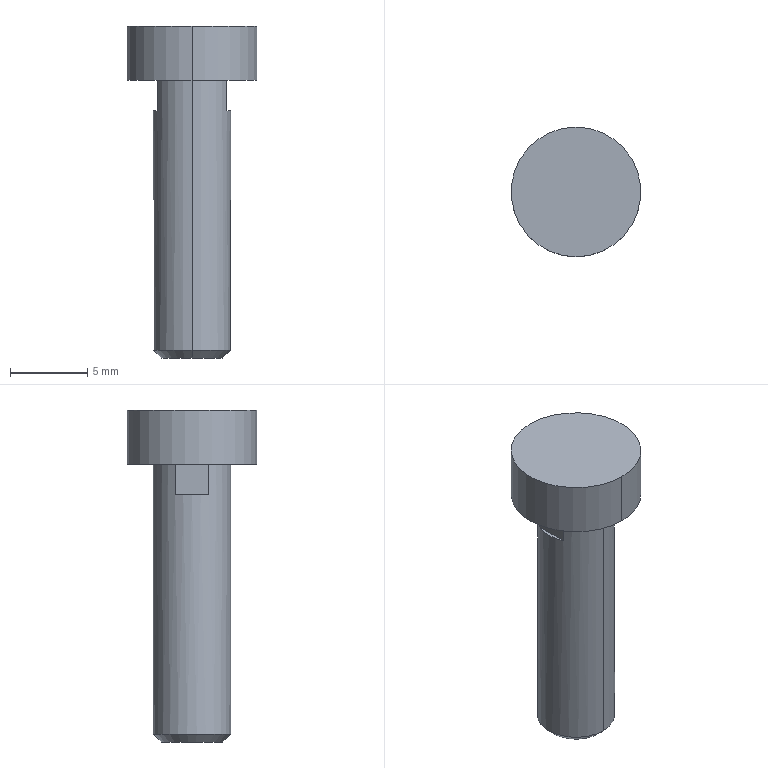Part | STEP file | M5 screw_default | 1 solid | 13 faces | box 8.4 x 8.4 x 21.5 mm | volume 544.09 mm3 | plane 7 | cylinder 4 | cone 2 | commonest cylinder face diameters 5 x2 8.4 x2
STEP:
#1=CARTESIAN_POINT('',(0.,0.,0.));
#2=DIRECTION('',(0.,0.,1.));
#3=DIRECTION('',(1.,0.,0.));
#4=AXIS2_PLACEMENT_3D('',#1,#2,#3);
#5=CARTESIAN_POINT('',(0.,2.,-3.));
#6=VERTEX_POINT('',#5);
#7=CARTESIAN_POINT('',(0.,-2.,-3.));
#8=VERTEX_POINT('',#7);
#9=CARTESIAN_POINT('',(0.,0.,-3.));
#10=DIRECTION('',(0.,0.,-1.));
#11=DIRECTION('',(-1.,0.,0.));
#12=AXIS2_PLACEMENT_3D('',#9,#10,#11);
#13=CIRCLE('',#12,2.);
#14=CARTESIAN_POINT('',(0.,0.,-3.));
#15=DIRECTION('',(0.,0.,1.));
#16=DIRECTION('',(0.,-1.,0.));
#17=AXIS2_PLACEMENT_3D('',#14,#15,#16);
#18=CONICAL_SURFACE('',#17,2.,0.7854);
#19=CARTESIAN_POINT('',(4.712,0.));
#20=DIRECTION('',(-1.,0.));
#21=VECTOR('',#20,1.);
#22=LINE('',#19,#21);
#23=(GEOMETRIC_REPRESENTATION_CONTEXT(2)PARAMETRIC_REPRESENTATION_CONTEXT()REPRESENTATION_CONTEXT('',''));
#24=DEFINITIONAL_REPRESENTATION('',(#22),#23);
#25=PCURVE('',#18,#24);
#26=CARTESIAN_POINT('',(0.,0.,-3.));
#27=DIRECTION('',(0.,0.,-1.));
#28=DIRECTION('',(-1.,0.,0.));
#29=AXIS2_PLACEMENT_3D('',#26,#27,#28);
#30=PLANE('',#29);
#31=CARTESIAN_POINT('',(0.,0.));
#32=DIRECTION('',(1.,0.));
#33=AXIS2_PLACEMENT_2D('',#31,#32);
#34=CIRCLE('',#33,2.);
#35=(GEOMETRIC_REPRESENTATION_CONTEXT(2)PARAMETRIC_REPRESENTATION_CONTEXT()REPRESENTATION_CONTEXT('',''));
#36=DEFINITIONAL_REPRESENTATION('',(#34),#35);
#37=PCURVE('',#30,#36);
#38=SURFACE_CURVE('',#13,(#25,#37),.PCURVE_S1.);
#39=EDGE_CURVE('',#6,#8,#38,.T.);
#40=ORIENTED_EDGE('',*,*,#39,.F.);
#41=CARTESIAN_POINT('',(0.,2.5,-2.5));
#42=VERTEX_POINT('',#41);
#43=CARTESIAN_POINT('',(0.,2.,-3.));
#44=DIRECTION('',(0.,0.7071,0.7071));
#45=VECTOR('',#44,1.);
#46=LINE('',#43,#45);
#47=CARTESIAN_POINT('',(3.142,0.));
#48=DIRECTION('',(0.,1.));
#49=VECTOR('',#48,1.);
#50=LINE('',#47,#49);
#51=(GEOMETRIC_REPRESENTATION_CONTEXT(2)PARAMETRIC_REPRESENTATION_CONTEXT()REPRESENTATION_CONTEXT('',''));
#52=DEFINITIONAL_REPRESENTATION('',(#50),#51);
#53=PCURVE('',#18,#52);
#54=CARTESIAN_POINT('',(0.,0.,-3.));
#55=DIRECTION('',(0.,0.,1.));
#56=DIRECTION('',(0.,-1.,0.));
#57=AXIS2_PLACEMENT_3D('',#54,#55,#56);
#58=CONICAL_SURFACE('',#57,2.,0.7854);
#59=CARTESIAN_POINT('',(3.142,0.));
#60=DIRECTION('',(0.,1.));
#61=VECTOR('',#60,1.);
#62=LINE('',#59,#61);
#63=(GEOMETRIC_REPRESENTATION_CONTEXT(2)PARAMETRIC_REPRESENTATION_CONTEXT()REPRESENTATION_CONTEXT('',''));
#64=DEFINITIONAL_REPRESENTATION('',(#62),#63);
#65=PCURVE('',#58,#64);
#66=SURFACE_CURVE('',#46,(#53,#65),.PCURVE_S1.);
#67=EDGE_CURVE('',#6,#42,#66,.T.);
#68=ORIENTED_EDGE('',*,*,#67,.T.);
#69=CARTESIAN_POINT('',(0.,-2.5,-2.5));
#70=VERTEX_POINT('',#69);
#71=CARTESIAN_POINT('',(0.,0.,-2.5));
#72=DIRECTION('',(0.,0.,1.));
#73=DIRECTION('',(0.,1.,0.));
#74=AXIS2_PLACEMENT_3D('',#71,#72,#73);
#75=CIRCLE('',#74,2.5);
#76=CARTESIAN_POINT('',(-3.142,0.5));
#77=DIRECTION('',(1.,0.));
#78=VECTOR('',#77,1.);
#79=LINE('',#76,#78);
#80=(GEOMETRIC_REPRESENTATION_CONTEXT(2)PARAMETRIC_REPRESENTATION_CONTEXT()REPRESENTATION_CONTEXT('',''));
#81=DEFINITIONAL_REPRESENTATION('',(#79),#80);
#82=PCURVE('',#18,#81);
#83=CARTESIAN_POINT('',(0.,0.,15.));
#84=DIRECTION('',(0.,0.,-1.));
#85=DIRECTION('',(0.,1.,0.));
#86=AXIS2_PLACEMENT_3D('',#83,#84,#85);
#87=CYLINDRICAL_SURFACE('',#86,2.5);
#88=CARTESIAN_POINT('',(6.283,17.5));
#89=DIRECTION('',(-1.,0.));
#90=VECTOR('',#89,1.);
#91=LINE('',#88,#90);
#92=(GEOMETRIC_REPRESENTATION_CONTEXT(2)PARAMETRIC_REPRESENTATION_CONTEXT()REPRESENTATION_CONTEXT('',''));
#93=DEFINITIONAL_REPRESENTATION('',(#91),#92);
#94=PCURVE('',#87,#93);
#95=SURFACE_CURVE('',#75,(#82,#94),.PCURVE_S1.);
#96=EDGE_CURVE('',#70,#42,#95,.T.);
#97=ORIENTED_EDGE('',*,*,#96,.F.);
#98=CARTESIAN_POINT('',(0.,-2.,-3.));
#99=DIRECTION('',(0.,-0.7071,0.7071));
#100=VECTOR('',#99,1.);
#101=LINE('',#98,#100);
#102=CARTESIAN_POINT('',(0.,0.));
#103=DIRECTION('',(0.,1.));
#104=VECTOR('',#103,1.);
#105=LINE('',#102,#104);
#106=(GEOMETRIC_REPRESENTATION_CONTEXT(2)PARAMETRIC_REPRESENTATION_CONTEXT()REPRESENTATION_CONTEXT('',''));
#107=DEFINITIONAL_REPRESENTATION('',(#105),#106);
#108=PCURVE('',#18,#107);
#109=CARTESIAN_POINT('',(6.283,0.));
#110=DIRECTION('',(0.,1.));
#111=VECTOR('',#110,1.);
#112=LINE('',#109,#111);
#113=(GEOMETRIC_REPRESENTATION_CONTEXT(2)PARAMETRIC_REPRESENTATION_CONTEXT()REPRESENTATION_CONTEXT('',''));
#114=DEFINITIONAL_REPRESENTATION('',(#112),#113);
#115=PCURVE('',#58,#114);
#116=SURFACE_CURVE('',#101,(#108,#115),.PCURVE_S1.);
#117=EDGE_CURVE('',#8,#70,#116,.T.);
#118=ORIENTED_EDGE('',*,*,#117,.F.);
#119=EDGE_LOOP('',(#40,#68,#97,#118));
#120=FACE_BOUND('',#119,.T.);
#121=ADVANCED_FACE('',(#120),#18,.T.);
#122=CARTESIAN_POINT('',(0.,-2.5,15.));
#123=VERTEX_POINT('',#122);
#124=CARTESIAN_POINT('',(2.25,-1.09,15.));
#125=VERTEX_POINT('',#124);
#126=CARTESIAN_POINT('',(0.,0.,15.));
#127=DIRECTION('',(0.,0.,1.));
#128=DIRECTION('',(0.,1.,0.));
#129=AXIS2_PLACEMENT_3D('',#126,#127,#128);
#130=CIRCLE('',#129,2.5);
#131=CARTESIAN_POINT('',(6.283,0.));
#132=DIRECTION('',(-1.,0.));
#133=VECTOR('',#132,1.);
#134=LINE('',#131,#133);
#135=(GEOMETRIC_REPRESENTATION_CONTEXT(2)PARAMETRIC_REPRESENTATION_CONTEXT()REPRESENTATION_CONTEXT('',''));
#136=DEFINITIONAL_REPRESENTATION('',(#134),#135);
#137=PCURVE('',#87,#136);
#138=CARTESIAN_POINT('',(-4.25,-4.25,15.));
#139=DIRECTION('',(0.,0.,1.));
#140=DIRECTION('',(1.,0.,0.));
#141=AXIS2_PLACEMENT_3D('',#138,#139,#140);
#142=PLANE('',#141);
#143=CARTESIAN_POINT('',(4.25,4.25));
#144=DIRECTION('',(0.,1.));
#145=AXIS2_PLACEMENT_2D('',#143,#144);
#146=CIRCLE('',#145,2.5);
#147=(GEOMETRIC_REPRESENTATION_CONTEXT(2)PARAMETRIC_REPRESENTATION_CONTEXT()REPRESENTATION_CONTEXT('',''));
#148=DEFINITIONAL_REPRESENTATION('',(#146),#147);
#149=PCURVE('',#142,#148);
#150=SURFACE_CURVE('',#130,(#137,#149),.PCURVE_S1.);
#151=EDGE_CURVE('',#123,#125,#150,.T.);
#152=ORIENTED_EDGE('',*,*,#151,.F.);
#153=CARTESIAN_POINT('',(0.,-2.5,15.));
#154=DIRECTION('',(0.,0.,-1.));
#155=VECTOR('',#154,1.);
#156=LINE('',#153,#155);
#157=CARTESIAN_POINT('',(3.142,0.));
#158=DIRECTION('',(0.,1.));
#159=VECTOR('',#158,1.);
#160=LINE('',#157,#159);
#161=(GEOMETRIC_REPRESENTATION_CONTEXT(2)PARAMETRIC_REPRESENTATION_CONTEXT()REPRESENTATION_CONTEXT('',''));
#162=DEFINITIONAL_REPRESENTATION('',(#160),#161);
#163=PCURVE('',#87,#162);
#164=CARTESIAN_POINT('',(0.,0.,15.));
#165=DIRECTION('',(0.,0.,-1.));
#166=DIRECTION('',(0.,1.,0.));
#167=AXIS2_PLACEMENT_3D('',#164,#165,#166);
#168=CYLINDRICAL_SURFACE('',#167,2.5);
#169=CARTESIAN_POINT('',(3.142,0.));
#170=DIRECTION('',(0.,1.));
#171=VECTOR('',#170,1.);
#172=LINE('',#169,#171);
#173=(GEOMETRIC_REPRESENTATION_CONTEXT(2)PARAMETRIC_REPRESENTATION_CONTEXT()REPRESENTATION_CONTEXT('',''));
#174=DEFINITIONAL_REPRESENTATION('',(#172),#173);
#175=PCURVE('',#168,#174);
#176=SURFACE_CURVE('',#156,(#163,#175),.PCURVE_S1.);
#177=EDGE_CURVE('',#123,#70,#176,.T.);
#178=ORIENTED_EDGE('',*,*,#177,.T.);
#179=ORIENTED_EDGE('',*,*,#96,.T.);
#180=CARTESIAN_POINT('',(0.,2.5,15.));
#181=VERTEX_POINT('',#180);
#182=CARTESIAN_POINT('',(0.,2.5,15.));
#183=DIRECTION('',(0.,0.,-1.));
#184=VECTOR('',#183,1.);
#185=LINE('',#182,#184);
#186=CARTESIAN_POINT('',(0.,0.));
#187=DIRECTION('',(0.,1.));
#188=VECTOR('',#187,1.);
#189=LINE('',#186,#188);
#190=(GEOMETRIC_REPRESENTATION_CONTEXT(2)PARAMETRIC_REPRESENTATION_CONTEXT()REPRESENTATION_CONTEXT('',''));
#191=DEFINITIONAL_REPRESENTATION('',(#189),#190);
#192=PCURVE('',#87,#191);
#193=CARTESIAN_POINT('',(6.283,0.));
#194=DIRECTION('',(0.,1.));
#195=VECTOR('',#194,1.);
#196=LINE('',#193,#195);
#197=(GEOMETRIC_REPRESENTATION_CONTEXT(2)PARAMETRIC_REPRESENTATION_CONTEXT()REPRESENTATION_CONTEXT('',''));
#198=DEFINITIONAL_REPRESENTATION('',(#196),#197);
#199=PCURVE('',#168,#198);
#200=SURFACE_CURVE('',#185,(#192,#199),.PCURVE_S1.);
#201=EDGE_CURVE('',#181,#42,#200,.T.);
#202=ORIENTED_EDGE('',*,*,#201,.F.);
#203=CARTESIAN_POINT('',(2.25,1.09,15.));
#204=VERTEX_POINT('',#203);
#205=CARTESIAN_POINT('',(0.,0.,15.));
#206=DIRECTION('',(0.,0.,1.));
#207=DIRECTION('',(0.,1.,0.));
#208=AXIS2_PLACEMENT_3D('',#205,#206,#207);
#209=CIRCLE('',#208,2.5);
#210=CARTESIAN_POINT('',(6.283,0.));
#211=DIRECTION('',(-1.,0.));
#212=VECTOR('',#211,1.);
#213=LINE('',#210,#212);
#214=(GEOMETRIC_REPRESENTATION_CONTEXT(2)PARAMETRIC_REPRESENTATION_CONTEXT()REPRESENTATION_CONTEXT('',''));
#215=DEFINITIONAL_REPRESENTATION('',(#213),#214);
#216=PCURVE('',#87,#215);
#217=CARTESIAN_POINT('',(4.25,4.25));
#218=DIRECTION('',(0.,1.));
#219=AXIS2_PLACEMENT_2D('',#217,#218);
#220=CIRCLE('',#219,2.5);
#221=(GEOMETRIC_REPRESENTATION_CONTEXT(2)PARAMETRIC_REPRESENTATION_CONTEXT()REPRESENTATION_CONTEXT('',''));
#222=DEFINITIONAL_REPRESENTATION('',(#220),#221);
#223=PCURVE('',#142,#222);
#224=SURFACE_CURVE('',#209,(#216,#223),.PCURVE_S1.);
#225=EDGE_CURVE('',#204,#181,#224,.T.);
#226=ORIENTED_EDGE('',*,*,#225,.F.);
#227=CARTESIAN_POINT('',(2.25,1.09,13.));
#228=VERTEX_POINT('',#227);
#229=CARTESIAN_POINT('',(2.25,1.09,15.));
#230=DIRECTION('',(0.,0.,-1.));
#231=VECTOR('',#230,1.);
#232=LINE('',#229,#231);
#233=CARTESIAN_POINT('',(1.12,0.));
#234=DIRECTION('',(0.,1.));
#235=VECTOR('',#234,1.);
#236=LINE('',#233,#235);
#237=(GEOMETRIC_REPRESENTATION_CONTEXT(2)PARAMETRIC_REPRESENTATION_CONTEXT()REPRESENTATION_CONTEXT('',''));
#238=DEFINITIONAL_REPRESENTATION('',(#236),#237);
#239=PCURVE('',#87,#238);
#240=CARTESIAN_POINT('',(2.25,-9.,15.));
#241=DIRECTION('',(-1.,0.,0.));
#242=DIRECTION('',(0.,0.,1.));
#243=AXIS2_PLACEMENT_3D('',#240,#241,#242);
#244=PLANE('',#243);
#245=CARTESIAN_POINT('',(0.,10.09));
#246=DIRECTION('',(-1.,0.));
#247=VECTOR('',#246,1.);
#248=LINE('',#245,#247);
#249=(GEOMETRIC_REPRESENTATION_CONTEXT(2)PARAMETRIC_REPRESENTATION_CONTEXT()REPRESENTATION_CONTEXT('',''));
#250=DEFINITIONAL_REPRESENTATION('',(#248),#249);
#251=PCURVE('',#244,#250);
#252=SURFACE_CURVE('',#232,(#239,#251),.PCURVE_S1.);
#253=EDGE_CURVE('',#204,#228,#252,.T.);
#254=ORIENTED_EDGE('',*,*,#253,.T.);
#255=CARTESIAN_POINT('',(2.25,-1.09,13.));
#256=VERTEX_POINT('',#255);
#257=CARTESIAN_POINT('',(0.,0.,13.));
#258=DIRECTION('',(0.,0.,-1.));
#259=DIRECTION('',(-1.,0.,0.));
#260=AXIS2_PLACEMENT_3D('',#257,#258,#259);
#261=CIRCLE('',#260,2.5);
#262=CARTESIAN_POINT('',(-1.571,2.));
#263=DIRECTION('',(1.,0.));
#264=VECTOR('',#263,1.);
#265=LINE('',#262,#264);
#266=(GEOMETRIC_REPRESENTATION_CONTEXT(2)PARAMETRIC_REPRESENTATION_CONTEXT()REPRESENTATION_CONTEXT('',''));
#267=DEFINITIONAL_REPRESENTATION('',(#265),#266);
#268=PCURVE('',#87,#267);
#269=CARTESIAN_POINT('',(3.25,-9.,13.));
#270=DIRECTION('',(0.,0.,-1.));
#271=DIRECTION('',(-1.,0.,0.));
#272=AXIS2_PLACEMENT_3D('',#269,#270,#271);
#273=PLANE('',#272);
#274=CARTESIAN_POINT('',(3.25,9.));
#275=DIRECTION('',(1.,0.));
#276=AXIS2_PLACEMENT_2D('',#274,#275);
#277=CIRCLE('',#276,2.5);
#278=(GEOMETRIC_REPRESENTATION_CONTEXT(2)PARAMETRIC_REPRESENTATION_CONTEXT()REPRESENTATION_CONTEXT('',''));
#279=DEFINITIONAL_REPRESENTATION('',(#277),#278);
#280=PCURVE('',#273,#279);
#281=SURFACE_CURVE('',#261,(#268,#280),.PCURVE_S1.);
#282=EDGE_CURVE('',#228,#256,#281,.T.);
#283=ORIENTED_EDGE('',*,*,#282,.T.);
#284=CARTESIAN_POINT('',(2.25,-1.09,15.));
#285=DIRECTION('',(0.,0.,1.));
#286=VECTOR('',#285,1.);
#287=LINE('',#284,#286);
#288=CARTESIAN_POINT('',(2.022,0.));
#289=DIRECTION('',(0.,-1.));
#290=VECTOR('',#289,1.);
#291=LINE('',#288,#290);
#292=(GEOMETRIC_REPRESENTATION_CONTEXT(2)PARAMETRIC_REPRESENTATION_CONTEXT()REPRESENTATION_CONTEXT('',''));
#293=DEFINITIONAL_REPRESENTATION('',(#291),#292);
#294=PCURVE('',#87,#293);
#295=CARTESIAN_POINT('',(0.,7.91));
#296=DIRECTION('',(1.,0.));
#297=VECTOR('',#296,1.);
#298=LINE('',#295,#297);
#299=(GEOMETRIC_REPRESENTATION_CONTEXT(2)PARAMETRIC_REPRESENTATION_CONTEXT()REPRESENTATION_CONTEXT('',''));
#300=DEFINITIONAL_REPRESENTATION('',(#298),#299);
#301=PCURVE('',#244,#300);
#302=SURFACE_CURVE('',#287,(#294,#301),.PCURVE_S1.);
#303=EDGE_CURVE('',#256,#125,#302,.T.);
#304=ORIENTED_EDGE('',*,*,#303,.T.);
#305=EDGE_LOOP('',(#152,#178,#179,#202,#226,#254,#283,#304));
#306=FACE_BOUND('',#305,.T.);
#307=ADVANCED_FACE('',(#306),#87,.T.);
#308=CARTESIAN_POINT('',(0.,-4.2,18.5));
#309=VERTEX_POINT('',#308);
#310=CARTESIAN_POINT('',(0.,4.2,18.5));
#311=VERTEX_POINT('',#310);
#312=CARTESIAN_POINT('',(0.,0.,18.5));
#313=DIRECTION('',(0.,0.,1.));
#314=DIRECTION('',(0.,1.,0.));
#315=AXIS2_PLACEMENT_3D('',#312,#313,#314);
#316=CIRCLE('',#315,4.2);
#317=CARTESIAN_POINT('',(0.,0.,18.5));
#318=DIRECTION('',(0.,0.,-1.));
#319=DIRECTION('',(0.,1.,0.));
#320=AXIS2_PLACEMENT_3D('',#317,#318,#319);
#321=CYLINDRICAL_SURFACE('',#320,4.2);
#322=CARTESIAN_POINT('',(6.283,0.));
#323=DIRECTION('',(-1.,0.));
#324=VECTOR('',#323,1.);
#325=LINE('',#322,#324);
#326=(GEOMETRIC_REPRESENTATION_CONTEXT(2)PARAMETRIC_REPRESENTATION_CONTEXT()REPRESENTATION_CONTEXT('',''));
#327=DEFINITIONAL_REPRESENTATION('',(#325),#326);
#328=PCURVE('',#321,#327);
#329=CARTESIAN_POINT('',(-4.25,-4.25,18.5));
#330=DIRECTION('',(0.,0.,1.));
#331=DIRECTION('',(1.,0.,0.));
#332=AXIS2_PLACEMENT_3D('',#329,#330,#331);
#333=PLANE('',#332);
#334=CARTESIAN_POINT('',(4.25,4.25));
#335=DIRECTION('',(0.,1.));
#336=AXIS2_PLACEMENT_2D('',#334,#335);
#337=CIRCLE('',#336,4.2);
#338=(GEOMETRIC_REPRESENTATION_CONTEXT(2)PARAMETRIC_REPRESENTATION_CONTEXT()REPRESENTATION_CONTEXT('',''));
#339=DEFINITIONAL_REPRESENTATION('',(#337),#338);
#340=PCURVE('',#333,#339);
#341=SURFACE_CURVE('',#316,(#328,#340),.PCURVE_S1.);
#342=EDGE_CURVE('',#309,#311,#341,.T.);
#343=ORIENTED_EDGE('',*,*,#342,.F.);
#344=CARTESIAN_POINT('',(0.,-4.2,15.));
#345=VERTEX_POINT('',#344);
#346=CARTESIAN_POINT('',(0.,-4.2,18.5));
#347=DIRECTION('',(0.,0.,-1.));
#348=VECTOR('',#347,1.);
#349=LINE('',#346,#348);
#350=CARTESIAN_POINT('',(3.142,0.));
#351=DIRECTION('',(0.,1.));
#352=VECTOR('',#351,1.);
#353=LINE('',#350,#352);
#354=(GEOMETRIC_REPRESENTATION_CONTEXT(2)PARAMETRIC_REPRESENTATION_CONTEXT()REPRESENTATION_CONTEXT('',''));
#355=DEFINITIONAL_REPRESENTATION('',(#353),#354);
#356=PCURVE('',#321,#355);
#357=CARTESIAN_POINT('',(0.,0.,18.5));
#358=DIRECTION('',(0.,0.,-1.));
#359=DIRECTION('',(0.,1.,0.));
#360=AXIS2_PLACEMENT_3D('',#357,#358,#359);
#361=CYLINDRICAL_SURFACE('',#360,4.2);
#362=CARTESIAN_POINT('',(3.142,0.));
#363=DIRECTION('',(0.,1.));
#364=VECTOR('',#363,1.);
#365=LINE('',#362,#364);
#366=(GEOMETRIC_REPRESENTATION_CONTEXT(2)PARAMETRIC_REPRESENTATION_CONTEXT()REPRESENTATION_CONTEXT('',''));
#367=DEFINITIONAL_REPRESENTATION('',(#365),#366);
#368=PCURVE('',#361,#367);
#369=SURFACE_CURVE('',#349,(#356,#368),.PCURVE_S1.);
#370=EDGE_CURVE('',#309,#345,#369,.T.);
#371=ORIENTED_EDGE('',*,*,#370,.T.);
#372=CARTESIAN_POINT('',(0.,4.2,15.));
#373=VERTEX_POINT('',#372);
#374=CARTESIAN_POINT('',(0.,0.,15.));
#375=DIRECTION('',(0.,0.,1.));
#376=DIRECTION('',(0.,1.,0.));
#377=AXIS2_PLACEMENT_3D('',#374,#375,#376);
#378=CIRCLE('',#377,4.2);
#379=CARTESIAN_POINT('',(6.283,3.5));
#380=DIRECTION('',(-1.,0.));
#381=VECTOR('',#380,1.);
#382=LINE('',#379,#381);
#383=(GEOMETRIC_REPRESENTATION_CONTEXT(2)PARAMETRIC_REPRESENTATION_CONTEXT()REPRESENTATION_CONTEXT('',''));
#384=DEFINITIONAL_REPRESENTATION('',(#382),#383);
#385=PCURVE('',#321,#384);
#386=CARTESIAN_POINT('',(4.25,4.25));
#387=DIRECTION('',(0.,1.));
#388=AXIS2_PLACEMENT_2D('',#386,#387);
#389=CIRCLE('',#388,4.2);
#390=(GEOMETRIC_REPRESENTATION_CONTEXT(2)PARAMETRIC_REPRESENTATION_CONTEXT()REPRESENTATION_CONTEXT('',''));
#391=DEFINITIONAL_REPRESENTATION('',(#389),#390);
#392=PCURVE('',#142,#391);
#393=SURFACE_CURVE('',#378,(#385,#392),.PCURVE_S1.);
#394=EDGE_CURVE('',#345,#373,#393,.T.);
#395=ORIENTED_EDGE('',*,*,#394,.T.);
#396=CARTESIAN_POINT('',(0.,4.2,18.5));
#397=DIRECTION('',(0.,0.,-1.));
#398=VECTOR('',#397,1.);
#399=LINE('',#396,#398);
#400=CARTESIAN_POINT('',(0.,0.));
#401=DIRECTION('',(0.,1.));
#402=VECTOR('',#401,1.);
#403=LINE('',#400,#402);
#404=(GEOMETRIC_REPRESENTATION_CONTEXT(2)PARAMETRIC_REPRESENTATION_CONTEXT()REPRESENTATION_CONTEXT('',''));
#405=DEFINITIONAL_REPRESENTATION('',(#403),#404);
#406=PCURVE('',#321,#405);
#407=CARTESIAN_POINT('',(6.283,0.));
#408=DIRECTION('',(0.,1.));
#409=VECTOR('',#408,1.);
#410=LINE('',#407,#409);
#411=(GEOMETRIC_REPRESENTATION_CONTEXT(2)PARAMETRIC_REPRESENTATION_CONTEXT()REPRESENTATION_CONTEXT('',''));
#412=DEFINITIONAL_REPRESENTATION('',(#410),#411);
#413=PCURVE('',#361,#412);
#414=SURFACE_CURVE('',#399,(#406,#413),.PCURVE_S1.);
#415=EDGE_CURVE('',#311,#373,#414,.T.);
#416=ORIENTED_EDGE('',*,*,#415,.F.);
#417=EDGE_LOOP('',(#343,#371,#395,#416));
#418=FACE_BOUND('',#417,.T.);
#419=ADVANCED_FACE('',(#418),#321,.T.);
#420=ORIENTED_EDGE('',*,*,#177,.F.);
#421=CARTESIAN_POINT('',(-2.25,-1.09,15.));
#422=VERTEX_POINT('',#421);
#423=CARTESIAN_POINT('',(0.,0.,15.));
#424=DIRECTION('',(0.,0.,1.));
#425=DIRECTION('',(0.,1.,0.));
#426=AXIS2_PLACEMENT_3D('',#423,#424,#425);
#427=CIRCLE('',#426,2.5);
#428=CARTESIAN_POINT('',(6.283,0.));
#429=DIRECTION('',(-1.,0.));
#430=VECTOR('',#429,1.);
#431=LINE('',#428,#430);
#432=(GEOMETRIC_REPRESENTATION_CONTEXT(2)PARAMETRIC_REPRESENTATION_CONTEXT()REPRESENTATION_CONTEXT('',''));
#433=DEFINITIONAL_REPRESENTATION('',(#431),#432);
#434=PCURVE('',#168,#433);
#435=CARTESIAN_POINT('',(4.25,4.25));
#436=DIRECTION('',(0.,1.));
#437=AXIS2_PLACEMENT_2D('',#435,#436);
#438=CIRCLE('',#437,2.5);
#439=(GEOMETRIC_REPRESENTATION_CONTEXT(2)PARAMETRIC_REPRESENTATION_CONTEXT()REPRESENTATION_CONTEXT('',''));
#440=DEFINITIONAL_REPRESENTATION('',(#438),#439);
#441=PCURVE('',#142,#440);
#442=SURFACE_CURVE('',#427,(#434,#441),.PCURVE_S1.);
#443=EDGE_CURVE('',#422,#123,#442,.T.);
#444=ORIENTED_EDGE('',*,*,#443,.F.);
#445=CARTESIAN_POINT('',(-2.25,-1.09,13.));
#446=VERTEX_POINT('',#445);
#447=CARTESIAN_POINT('',(-2.25,-1.09,15.));
#448=DIRECTION('',(0.,0.,-1.));
#449=VECTOR('',#448,1.);
#450=LINE('',#447,#449);
#451=CARTESIAN_POINT('',(4.261,0.));
#452=DIRECTION('',(0.,1.));
#453=VECTOR('',#452,1.);
#454=LINE('',#451,#453);
#455=(GEOMETRIC_REPRESENTATION_CONTEXT(2)PARAMETRIC_REPRESENTATION_CONTEXT()REPRESENTATION_CONTEXT('',''));
#456=DEFINITIONAL_REPRESENTATION('',(#454),#455);
#457=PCURVE('',#168,#456);
#458=CARTESIAN_POINT('',(-2.25,-9.,15.));
#459=DIRECTION('',(1.,0.,0.));
#460=DIRECTION('',(0.,0.,-1.));
#461=AXIS2_PLACEMENT_3D('',#458,#459,#460);
#462=PLANE('',#461);
#463=CARTESIAN_POINT('',(0.,7.91));
#464=DIRECTION('',(1.,0.));
#465=VECTOR('',#464,1.);
#466=LINE('',#463,#465);
#467=(GEOMETRIC_REPRESENTATION_CONTEXT(2)PARAMETRIC_REPRESENTATION_CONTEXT()REPRESENTATION_CONTEXT('',''));
#468=DEFINITIONAL_REPRESENTATION('',(#466),#467);
#469=PCURVE('',#462,#468);
#470=SURFACE_CURVE('',#450,(#457,#469),.PCURVE_S1.);
#471=EDGE_CURVE('',#422,#446,#470,.T.);
#472=ORIENTED_EDGE('',*,*,#471,.T.);
#473=CARTESIAN_POINT('',(-2.25,1.09,13.));
#474=VERTEX_POINT('',#473);
#475=CARTESIAN_POINT('',(0.,0.,13.));
#476=DIRECTION('',(0.,0.,-1.));
#477=DIRECTION('',(-1.,0.,0.));
#478=AXIS2_PLACEMENT_3D('',#475,#476,#477);
#479=CIRCLE('',#478,2.5);
#480=CARTESIAN_POINT('',(-1.571,2.));
#481=DIRECTION('',(1.,0.));
#482=VECTOR('',#481,1.);
#483=LINE('',#480,#482);
#484=(GEOMETRIC_REPRESENTATION_CONTEXT(2)PARAMETRIC_REPRESENTATION_CONTEXT()REPRESENTATION_CONTEXT('',''));
#485=DEFINITIONAL_REPRESENTATION('',(#483),#484);
#486=PCURVE('',#168,#485);
#487=CARTESIAN_POINT('',(-3.25,-9.,13.));
#488=DIRECTION('',(0.,0.,-1.));
#489=DIRECTION('',(-1.,0.,0.));
#490=AXIS2_PLACEMENT_3D('',#487,#488,#489);
#491=PLANE('',#490);
#492=CARTESIAN_POINT('',(-3.25,9.));
#493=DIRECTION('',(1.,0.));
#494=AXIS2_PLACEMENT_2D('',#492,#493);
#495=CIRCLE('',#494,2.5);
#496=(GEOMETRIC_REPRESENTATION_CONTEXT(2)PARAMETRIC_REPRESENTATION_CONTEXT()REPRESENTATION_CONTEXT('',''));
#497=DEFINITIONAL_REPRESENTATION('',(#495),#496);
#498=PCURVE('',#491,#497);
#499=SURFACE_CURVE('',#479,(#486,#498),.PCURVE_S1.);
#500=EDGE_CURVE('',#446,#474,#499,.T.);
#501=ORIENTED_EDGE('',*,*,#500,.T.);
#502=CARTESIAN_POINT('',(-2.25,1.09,15.));
#503=VERTEX_POINT('',#502);
#504=CARTESIAN_POINT('',(-2.25,1.09,15.));
#505=DIRECTION('',(0.,0.,1.));
#506=VECTOR('',#505,1.);
#507=LINE('',#504,#506);
#508=CARTESIAN_POINT('',(5.163,0.));
#509=DIRECTION('',(0.,-1.));
#510=VECTOR('',#509,1.);
#511=LINE('',#508,#510);
#512=(GEOMETRIC_REPRESENTATION_CONTEXT(2)PARAMETRIC_REPRESENTATION_CONTEXT()REPRESENTATION_CONTEXT('',''));
#513=DEFINITIONAL_REPRESENTATION('',(#511),#512);
#514=PCURVE('',#168,#513);
#515=CARTESIAN_POINT('',(0.,10.09));
#516=DIRECTION('',(-1.,0.));
#517=VECTOR('',#516,1.);
#518=LINE('',#515,#517);
#519=(GEOMETRIC_REPRESENTATION_CONTEXT(2)PARAMETRIC_REPRESENTATION_CONTEXT()REPRESENTATION_CONTEXT('',''));
#520=DEFINITIONAL_REPRESENTATION('',(#518),#519);
#521=PCURVE('',#462,#520);
#522=SURFACE_CURVE('',#507,(#514,#521),.PCURVE_S1.);
#523=EDGE_CURVE('',#474,#503,#522,.T.);
#524=ORIENTED_EDGE('',*,*,#523,.T.);
#525=CARTESIAN_POINT('',(0.,0.,15.));
#526=DIRECTION('',(0.,0.,1.));
#527=DIRECTION('',(0.,1.,0.));
#528=AXIS2_PLACEMENT_3D('',#525,#526,#527);
#529=CIRCLE('',#528,2.5);
#530=CARTESIAN_POINT('',(6.283,0.));
#531=DIRECTION('',(-1.,0.));
#532=VECTOR('',#531,1.);
#533=LINE('',#530,#532);
#534=(GEOMETRIC_REPRESENTATION_CONTEXT(2)PARAMETRIC_REPRESENTATION_CONTEXT()REPRESENTATION_CONTEXT('',''));
#535=DEFINITIONAL_REPRESENTATION('',(#533),#534);
#536=PCURVE('',#168,#535);
#537=CARTESIAN_POINT('',(4.25,4.25));
#538=DIRECTION('',(0.,1.));
#539=AXIS2_PLACEMENT_2D('',#537,#538);
#540=CIRCLE('',#539,2.5);
#541=(GEOMETRIC_REPRESENTATION_CONTEXT(2)PARAMETRIC_REPRESENTATION_CONTEXT()REPRESENTATION_CONTEXT('',''));
#542=DEFINITIONAL_REPRESENTATION('',(#540),#541);
#543=PCURVE('',#142,#542);
#544=SURFACE_CURVE('',#529,(#536,#543),.PCURVE_S1.);
#545=EDGE_CURVE('',#181,#503,#544,.T.);
#546=ORIENTED_EDGE('',*,*,#545,.F.);
#547=ORIENTED_EDGE('',*,*,#201,.T.);
#548=CARTESIAN_POINT('',(0.,0.,-2.5));
#549=DIRECTION('',(0.,0.,1.));
#550=DIRECTION('',(0.,1.,0.));
#551=AXIS2_PLACEMENT_3D('',#548,#549,#550);
#552=CIRCLE('',#551,2.5);
#553=CARTESIAN_POINT('',(6.283,17.5));
#554=DIRECTION('',(-1.,0.));
#555=VECTOR('',#554,1.);
#556=LINE('',#553,#555);
#557=(GEOMETRIC_REPRESENTATION_CONTEXT(2)PARAMETRIC_REPRESENTATION_CONTEXT()REPRESENTATION_CONTEXT('',''));
#558=DEFINITIONAL_REPRESENTATION('',(#556),#557);
#559=PCURVE('',#168,#558);
#560=CARTESIAN_POINT('',(3.142,0.5));
#561=DIRECTION('',(1.,0.));
#562=VECTOR('',#561,1.);
#563=LINE('',#560,#562);
#564=(GEOMETRIC_REPRESENTATION_CONTEXT(2)PARAMETRIC_REPRESENTATION_CONTEXT()REPRESENTATION_CONTEXT('',''));
#565=DEFINITIONAL_REPRESENTATION('',(#563),#564);
#566=PCURVE('',#58,#565);
#567=SURFACE_CURVE('',#552,(#559,#566),.PCURVE_S1.);
#568=EDGE_CURVE('',#42,#70,#567,.T.);
#569=ORIENTED_EDGE('',*,*,#568,.T.);
#570=EDGE_LOOP('',(#420,#444,#472,#501,#524,#546,#547,#569));
#571=FACE_BOUND('',#570,.T.);
#572=ADVANCED_FACE('',(#571),#168,.T.);
#573=CARTESIAN_POINT('',(2.25,-9.,15.));
#574=DIRECTION('',(0.,1.,0.));
#575=VECTOR('',#574,1.);
#576=LINE('',#573,#575);
#577=CARTESIAN_POINT('',(6.5,-4.75));
#578=DIRECTION('',(0.,1.));
#579=VECTOR('',#578,1.);
#580=LINE('',#577,#579);
#581=(GEOMETRIC_REPRESENTATION_CONTEXT(2)PARAMETRIC_REPRESENTATION_CONTEXT()REPRESENTATION_CONTEXT('',''));
#582=DEFINITIONAL_REPRESENTATION('',(#580),#581);
#583=PCURVE('',#142,#582);
#584=CARTESIAN_POINT('',(0.,0.));
#585=DIRECTION('',(0.,1.));
#586=VECTOR('',#585,1.);
#587=LINE('',#584,#586);
#588=(GEOMETRIC_REPRESENTATION_CONTEXT(2)PARAMETRIC_REPRESENTATION_CONTEXT()REPRESENTATION_CONTEXT('',''));
#589=DEFINITIONAL_REPRESENTATION('',(#587),#588);
#590=PCURVE('',#244,#589);
#591=SURFACE_CURVE('',#576,(#583,#590),.PCURVE_S1.);
#592=EDGE_CURVE('',#125,#204,#591,.T.);
#593=ORIENTED_EDGE('',*,*,#592,.T.);
#594=ORIENTED_EDGE('',*,*,#225,.T.);
#595=ORIENTED_EDGE('',*,*,#545,.T.);
#596=CARTESIAN_POINT('',(-2.25,-9.,15.));
#597=DIRECTION('',(0.,1.,0.));
#598=VECTOR('',#597,1.);
#599=LINE('',#596,#598);
#600=CARTESIAN_POINT('',(2.,-4.75));
#601=DIRECTION('',(0.,1.));
#602=VECTOR('',#601,1.);
#603=LINE('',#600,#602);
#604=(GEOMETRIC_REPRESENTATION_CONTEXT(2)PARAMETRIC_REPRESENTATION_CONTEXT()REPRESENTATION_CONTEXT('',''));
#605=DEFINITIONAL_REPRESENTATION('',(#603),#604);
#606=PCURVE('',#142,#605);
#607=CARTESIAN_POINT('',(0.,0.));
#608=DIRECTION('',(0.,1.));
#609=VECTOR('',#608,1.);
#610=LINE('',#607,#609);
#611=(GEOMETRIC_REPRESENTATION_CONTEXT(2)PARAMETRIC_REPRESENTATION_CONTEXT()REPRESENTATION_CONTEXT('',''));
#612=DEFINITIONAL_REPRESENTATION('',(#610),#611);
#613=PCURVE('',#462,#612);
#614=SURFACE_CURVE('',#599,(#606,#613),.PCURVE_S1.);
#615=EDGE_CURVE('',#422,#503,#614,.T.);
#616=ORIENTED_EDGE('',*,*,#615,.F.);
#617=ORIENTED_EDGE('',*,*,#443,.T.);
#618=ORIENTED_EDGE('',*,*,#151,.T.);
#619=EDGE_LOOP('',(#593,#594,#595,#616,#617,#618));
#620=FACE_BOUND('',#619,.T.);
#621=CARTESIAN_POINT('',(0.,0.,15.));
#622=DIRECTION('',(0.,0.,1.));
#623=DIRECTION('',(0.,1.,0.));
#624=AXIS2_PLACEMENT_3D('',#621,#622,#623);
#625=CIRCLE('',#624,4.2);
#626=CARTESIAN_POINT('',(4.25,4.25));
#627=DIRECTION('',(0.,1.));
#628=AXIS2_PLACEMENT_2D('',#626,#627);
#629=CIRCLE('',#628,4.2);
#630=(GEOMETRIC_REPRESENTATION_CONTEXT(2)PARAMETRIC_REPRESENTATION_CONTEXT()REPRESENTATION_CONTEXT('',''));
#631=DEFINITIONAL_REPRESENTATION('',(#629),#630);
#632=PCURVE('',#142,#631);
#633=CARTESIAN_POINT('',(6.283,3.5));
#634=DIRECTION('',(-1.,0.));
#635=VECTOR('',#634,1.);
#636=LINE('',#633,#635);
#637=(GEOMETRIC_REPRESENTATION_CONTEXT(2)PARAMETRIC_REPRESENTATION_CONTEXT()REPRESENTATION_CONTEXT('',''));
#638=DEFINITIONAL_REPRESENTATION('',(#636),#637);
#639=PCURVE('',#361,#638);
#640=SURFACE_CURVE('',#625,(#632,#639),.PCURVE_S1.);
#641=EDGE_CURVE('',#373,#345,#640,.T.);
#642=ORIENTED_EDGE('',*,*,#641,.F.);
#643=ORIENTED_EDGE('',*,*,#394,.F.);
#644=EDGE_LOOP('',(#642,#643));
#645=FACE_BOUND('',#644,.T.);
#646=ADVANCED_FACE('',(#620,#645),#142,.F.);
#647=ORIENTED_EDGE('',*,*,#370,.F.);
#648=CARTESIAN_POINT('',(0.,0.,18.5));
#649=DIRECTION('',(0.,0.,1.));
#650=DIRECTION('',(0.,1.,0.));
#651=AXIS2_PLACEMENT_3D('',#648,#649,#650);
#652=CIRCLE('',#651,4.2);
#653=CARTESIAN_POINT('',(6.283,0.));
#654=DIRECTION('',(-1.,0.));
#655=VECTOR('',#654,1.);
#656=LINE('',#653,#655);
#657=(GEOMETRIC_REPRESENTATION_CONTEXT(2)PARAMETRIC_REPRESENTATION_CONTEXT()REPRESENTATION_CONTEXT('',''));
#658=DEFINITIONAL_REPRESENTATION('',(#656),#657);
#659=PCURVE('',#361,#658);
#660=CARTESIAN_POINT('',(4.25,4.25));
#661=DIRECTION('',(0.,1.));
#662=AXIS2_PLACEMENT_2D('',#660,#661);
#663=CIRCLE('',#662,4.2);
#664=(GEOMETRIC_REPRESENTATION_CONTEXT(2)PARAMETRIC_REPRESENTATION_CONTEXT()REPRESENTATION_CONTEXT('',''));
#665=DEFINITIONAL_REPRESENTATION('',(#663),#664);
#666=PCURVE('',#333,#665);
#667=SURFACE_CURVE('',#652,(#659,#666),.PCURVE_S1.);
#668=EDGE_CURVE('',#311,#309,#667,.T.);
#669=ORIENTED_EDGE('',*,*,#668,.F.);
#670=ORIENTED_EDGE('',*,*,#415,.T.);
#671=ORIENTED_EDGE('',*,*,#641,.T.);
#672=EDGE_LOOP('',(#647,#669,#670,#671));
#673=FACE_BOUND('',#672,.T.);
#674=ADVANCED_FACE('',(#673),#361,.T.);
#675=ORIENTED_EDGE('',*,*,#668,.T.);
#676=ORIENTED_EDGE('',*,*,#342,.T.);
#677=EDGE_LOOP('',(#675,#676));
#678=FACE_BOUND('',#677,.T.);
#679=ADVANCED_FACE('',(#678),#333,.T.);
#680=CARTESIAN_POINT('',(0.,0.,-3.));
#681=DIRECTION('',(0.,0.,-1.));
#682=DIRECTION('',(-1.,0.,0.));
#683=AXIS2_PLACEMENT_3D('',#680,#681,#682);
#684=CIRCLE('',#683,2.);
#685=CARTESIAN_POINT('',(0.,0.));
#686=DIRECTION('',(1.,0.));
#687=AXIS2_PLACEMENT_2D('',#685,#686);
#688=CIRCLE('',#687,2.);
#689=(GEOMETRIC_REPRESENTATION_CONTEXT(2)PARAMETRIC_REPRESENTATION_CONTEXT()REPRESENTATION_CONTEXT('',''));
#690=DEFINITIONAL_REPRESENTATION('',(#688),#689);
#691=PCURVE('',#30,#690);
#692=CARTESIAN_POINT('',(10.996,0.));
#693=DIRECTION('',(-1.,0.));
#694=VECTOR('',#693,1.);
#695=LINE('',#692,#694);
#696=(GEOMETRIC_REPRESENTATION_CONTEXT(2)PARAMETRIC_REPRESENTATION_CONTEXT()REPRESENTATION_CONTEXT('',''));
#697=DEFINITIONAL_REPRESENTATION('',(#695),#696);
#698=PCURVE('',#58,#697);
#699=SURFACE_CURVE('',#684,(#691,#698),.PCURVE_S1.);
#700=EDGE_CURVE('',#8,#6,#699,.T.);
#701=ORIENTED_EDGE('',*,*,#700,.T.);
#702=ORIENTED_EDGE('',*,*,#39,.T.);
#703=EDGE_LOOP('',(#701,#702));
#704=FACE_BOUND('',#703,.T.);
#705=ADVANCED_FACE('',(#704),#30,.T.);
#706=ORIENTED_EDGE('',*,*,#67,.F.);
#707=ORIENTED_EDGE('',*,*,#700,.F.);
#708=ORIENTED_EDGE('',*,*,#117,.T.);
#709=ORIENTED_EDGE('',*,*,#568,.F.);
#710=EDGE_LOOP('',(#706,#707,#708,#709));
#711=FACE_BOUND('',#710,.T.);
#712=ADVANCED_FACE('',(#711),#58,.T.);
#713=CARTESIAN_POINT('',(-2.25,-9.,13.));
#714=DIRECTION('',(0.,1.,0.));
#715=VECTOR('',#714,1.);
#716=LINE('',#713,#715);
#717=CARTESIAN_POINT('',(-1.,0.));
#718=DIRECTION('',(0.,1.));
#719=VECTOR('',#718,1.);
#720=LINE('',#717,#719);
#721=(GEOMETRIC_REPRESENTATION_CONTEXT(2)PARAMETRIC_REPRESENTATION_CONTEXT()REPRESENTATION_CONTEXT('',''));
#722=DEFINITIONAL_REPRESENTATION('',(#720),#721);
#723=PCURVE('',#491,#722);
#724=CARTESIAN_POINT('',(2.,0.));
#725=DIRECTION('',(0.,1.));
#726=VECTOR('',#725,1.);
#727=LINE('',#724,#726);
#728=(GEOMETRIC_REPRESENTATION_CONTEXT(2)PARAMETRIC_REPRESENTATION_CONTEXT()REPRESENTATION_CONTEXT('',''));
#729=DEFINITIONAL_REPRESENTATION('',(#727),#728);
#730=PCURVE('',#462,#729);
#731=SURFACE_CURVE('',#716,(#723,#730),.PCURVE_S1.);
#732=EDGE_CURVE('',#446,#474,#731,.T.);
#733=ORIENTED_EDGE('',*,*,#732,.T.);
#734=ORIENTED_EDGE('',*,*,#500,.F.);
#735=EDGE_LOOP('',(#733,#734));
#736=FACE_BOUND('',#735,.T.);
#737=ADVANCED_FACE('',(#736),#491,.F.);
#738=ORIENTED_EDGE('',*,*,#615,.T.);
#739=ORIENTED_EDGE('',*,*,#523,.F.);
#740=ORIENTED_EDGE('',*,*,#732,.F.);
#741=ORIENTED_EDGE('',*,*,#471,.F.);
#742=EDGE_LOOP('',(#738,#739,#740,#741));
#743=FACE_BOUND('',#742,.T.);
#744=ADVANCED_FACE('',(#743),#462,.F.);
#745=ORIENTED_EDGE('',*,*,#592,.F.);
#746=ORIENTED_EDGE('',*,*,#303,.F.);
#747=CARTESIAN_POINT('',(2.25,-9.,13.));
#748=DIRECTION('',(0.,1.,0.));
#749=VECTOR('',#748,1.);
#750=LINE('',#747,#749);
#751=CARTESIAN_POINT('',(-2.,0.));
#752=DIRECTION('',(0.,1.));
#753=VECTOR('',#752,1.);
#754=LINE('',#751,#753);
#755=(GEOMETRIC_REPRESENTATION_CONTEXT(2)PARAMETRIC_REPRESENTATION_CONTEXT()REPRESENTATION_CONTEXT('',''));
#756=DEFINITIONAL_REPRESENTATION('',(#754),#755);
#757=PCURVE('',#244,#756);
#758=CARTESIAN_POINT('',(1.,0.));
#759=DIRECTION('',(0.,1.));
#760=VECTOR('',#759,1.);
#761=LINE('',#758,#760);
#762=(GEOMETRIC_REPRESENTATION_CONTEXT(2)PARAMETRIC_REPRESENTATION_CONTEXT()REPRESENTATION_CONTEXT('',''));
#763=DEFINITIONAL_REPRESENTATION('',(#761),#762);
#764=PCURVE('',#273,#763);
#765=SURFACE_CURVE('',#750,(#757,#764),.PCURVE_S1.);
#766=EDGE_CURVE('',#256,#228,#765,.T.);
#767=ORIENTED_EDGE('',*,*,#766,.T.);
#768=ORIENTED_EDGE('',*,*,#253,.F.);
#769=EDGE_LOOP('',(#745,#746,#767,#768));
#770=FACE_BOUND('',#769,.T.);
#771=ADVANCED_FACE('',(#770),#244,.F.);
#772=ORIENTED_EDGE('',*,*,#766,.F.);
#773=ORIENTED_EDGE('',*,*,#282,.F.);
#774=EDGE_LOOP('',(#772,#773));
#775=FACE_BOUND('',#774,.T.);
#776=ADVANCED_FACE('',(#775),#273,.F.);
#777=CLOSED_SHELL('',(#121,#307,#419,#572,#646,#674,#679,#705,#712,#737,#744,#771,#776));
#778=MANIFOLD_SOLID_BREP('',#777);
#779=(LENGTH_UNIT()NAMED_UNIT(*)SI_UNIT(.MILLI.,.METRE.));
#780=UNCERTAINTY_MEASURE_WITH_UNIT(LENGTH_MEASURE(0.0000001),#779,'','');
#781=(NAMED_UNIT(*)PLANE_ANGLE_UNIT()SI_UNIT($,.RADIAN.));
#782=(NAMED_UNIT(*)SI_UNIT($,.STERADIAN.)SOLID_ANGLE_UNIT());
#783=(GEOMETRIC_REPRESENTATION_CONTEXT(3)GLOBAL_UNCERTAINTY_ASSIGNED_CONTEXT((#780))GLOBAL_UNIT_ASSIGNED_CONTEXT((#779,#781,#782))REPRESENTATION_CONTEXT('',''));
#784=ADVANCED_BREP_SHAPE_REPRESENTATION('',(#4,#778),#783);